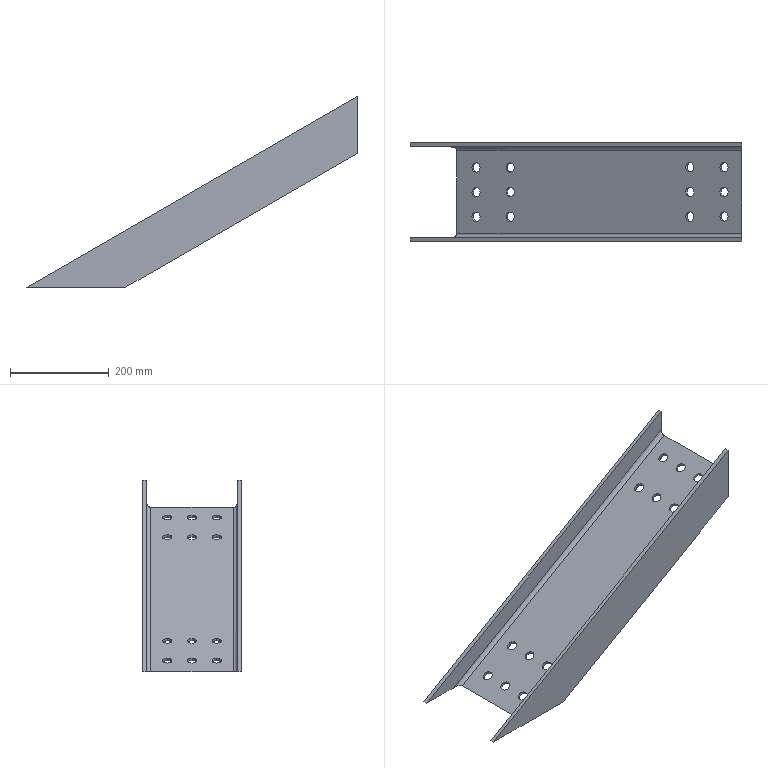Part | STEP file | 粉仓Diagonal Brace梁8_Default<As Machined> | 1 solid | 42 faces | box 671.577 x 200 x 387.735 mm | volume 1741466 mm3 | cylinder 28 | plane 14 | commonest cylinder face diameters 19 x24 16 x4